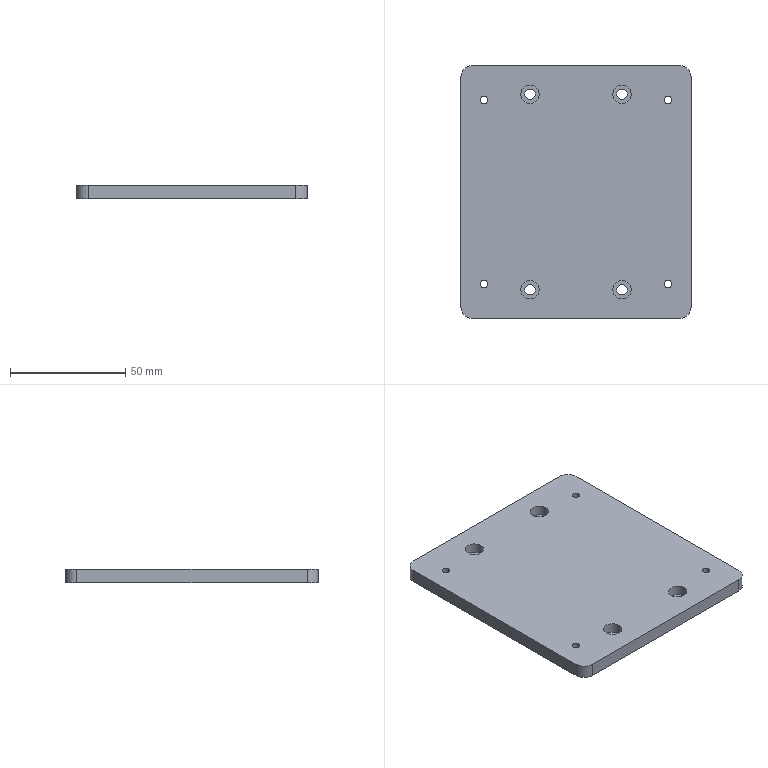Part | SolidWorks | features HoleWzd 2, Extrusion 1, Fillet 1 | 1 solid | 38 faces | box 100 x 110 x 6 mm | volume 64666 mm3 | cylinder 28 | plane 10 | commonest cylinder face diameters 3.3 x8 4.5 x8 8 x8 10 x4
STEP:
#1=CARTESIAN_POINT('',(-41.65,-40.,0.));
#2=VERTEX_POINT('',#1);
#3=CARTESIAN_POINT('',(-38.35,-40.,0.));
#4=VERTEX_POINT('',#3);
#5=CARTESIAN_POINT('',(-40.,-40.,0.));
#6=DIRECTION('',(0.,0.,1.));
#7=DIRECTION('',(1.,0.,0.));
#8=AXIS2_PLACEMENT_3D('',#5,#6,#7);
#9=CIRCLE('',#8,1.65);
#10=EDGE_CURVE('',#2,#4,#9,.T.);
#11=ORIENTED_EDGE('',*,*,#10,.F.);
#12=CARTESIAN_POINT('',(-41.65,-40.,6.));
#13=VERTEX_POINT('',#12);
#14=CARTESIAN_POINT('',(-41.65,-40.,6.));
#15=DIRECTION('',(0.,0.,1.));
#16=VECTOR('',#15,1000.);
#17=LINE('',#14,#16);
#18=EDGE_CURVE('',#2,#13,#17,.T.);
#19=ORIENTED_EDGE('',*,*,#18,.T.);
#20=CARTESIAN_POINT('',(-38.35,-40.,6.));
#21=VERTEX_POINT('',#20);
#22=CARTESIAN_POINT('',(-40.,-40.,6.));
#23=DIRECTION('',(0.,0.,1.));
#24=DIRECTION('',(1.,0.,0.));
#25=AXIS2_PLACEMENT_3D('',#22,#23,#24);
#26=CIRCLE('',#25,1.65);
#27=EDGE_CURVE('',#13,#21,#26,.T.);
#28=ORIENTED_EDGE('',*,*,#27,.T.);
#29=CARTESIAN_POINT('',(-38.35,-40.,6.));
#30=DIRECTION('',(0.,0.,1.));
#31=VECTOR('',#30,1000.);
#32=LINE('',#29,#31);
#33=EDGE_CURVE('',#4,#21,#32,.T.);
#34=ORIENTED_EDGE('',*,*,#33,.F.);
#35=EDGE_LOOP('',(#11,#19,#28,#34));
#36=FACE_OUTER_BOUND('',#35,.T.);
#37=CARTESIAN_POINT('',(-40.,-40.,6.));
#38=DIRECTION('',(0.,0.,1.));
#39=DIRECTION('',(1.,0.,0.));
#40=AXIS2_PLACEMENT_3D('',#37,#38,#39);
#41=CYLINDRICAL_SURFACE('',#40,1.65);
#42=ADVANCED_FACE('',(#36),#41,.F.);
#43=CARTESIAN_POINT('',(38.35,-40.,0.));
#44=VERTEX_POINT('',#43);
#45=CARTESIAN_POINT('',(41.65,-40.,0.));
#46=VERTEX_POINT('',#45);
#47=CARTESIAN_POINT('',(40.,-40.,0.));
#48=DIRECTION('',(0.,0.,1.));
#49=DIRECTION('',(1.,0.,0.));
#50=AXIS2_PLACEMENT_3D('',#47,#48,#49);
#51=CIRCLE('',#50,1.65);
#52=EDGE_CURVE('',#44,#46,#51,.T.);
#53=ORIENTED_EDGE('',*,*,#52,.F.);
#54=CARTESIAN_POINT('',(38.35,-40.,6.));
#55=VERTEX_POINT('',#54);
#56=CARTESIAN_POINT('',(38.35,-40.,6.));
#57=DIRECTION('',(0.,0.,1.));
#58=VECTOR('',#57,1000.);
#59=LINE('',#56,#58);
#60=EDGE_CURVE('',#44,#55,#59,.T.);
#61=ORIENTED_EDGE('',*,*,#60,.T.);
#62=CARTESIAN_POINT('',(41.65,-40.,6.));
#63=VERTEX_POINT('',#62);
#64=CARTESIAN_POINT('',(40.,-40.,6.));
#65=DIRECTION('',(0.,0.,1.));
#66=DIRECTION('',(1.,0.,0.));
#67=AXIS2_PLACEMENT_3D('',#64,#65,#66);
#68=CIRCLE('',#67,1.65);
#69=EDGE_CURVE('',#55,#63,#68,.T.);
#70=ORIENTED_EDGE('',*,*,#69,.T.);
#71=CARTESIAN_POINT('',(41.65,-40.,6.));
#72=DIRECTION('',(0.,0.,1.));
#73=VECTOR('',#72,1000.);
#74=LINE('',#71,#73);
#75=EDGE_CURVE('',#46,#63,#74,.T.);
#76=ORIENTED_EDGE('',*,*,#75,.F.);
#77=EDGE_LOOP('',(#53,#61,#70,#76));
#78=FACE_OUTER_BOUND('',#77,.T.);
#79=CARTESIAN_POINT('',(40.,-40.,6.));
#80=DIRECTION('',(0.,0.,1.));
#81=DIRECTION('',(1.,0.,0.));
#82=AXIS2_PLACEMENT_3D('',#79,#80,#81);
#83=CYLINDRICAL_SURFACE('',#82,1.65);
#84=ADVANCED_FACE('',(#78),#83,.F.);
#85=CARTESIAN_POINT('',(38.35,40.,0.));
#86=VERTEX_POINT('',#85);
#87=CARTESIAN_POINT('',(41.65,40.,0.));
#88=VERTEX_POINT('',#87);
#89=CARTESIAN_POINT('',(40.,40.,0.));
#90=DIRECTION('',(0.,0.,1.));
#91=DIRECTION('',(1.,0.,0.));
#92=AXIS2_PLACEMENT_3D('',#89,#90,#91);
#93=CIRCLE('',#92,1.65);
#94=EDGE_CURVE('',#86,#88,#93,.T.);
#95=ORIENTED_EDGE('',*,*,#94,.F.);
#96=CARTESIAN_POINT('',(38.35,40.,6.));
#97=VERTEX_POINT('',#96);
#98=CARTESIAN_POINT('',(38.35,40.,6.));
#99=DIRECTION('',(0.,0.,1.));
#100=VECTOR('',#99,1000.);
#101=LINE('',#98,#100);
#102=EDGE_CURVE('',#86,#97,#101,.T.);
#103=ORIENTED_EDGE('',*,*,#102,.T.);
#104=CARTESIAN_POINT('',(41.65,40.,6.));
#105=VERTEX_POINT('',#104);
#106=CARTESIAN_POINT('',(40.,40.,6.));
#107=DIRECTION('',(0.,0.,1.));
#108=DIRECTION('',(1.,0.,0.));
#109=AXIS2_PLACEMENT_3D('',#106,#107,#108);
#110=CIRCLE('',#109,1.65);
#111=EDGE_CURVE('',#97,#105,#110,.T.);
#112=ORIENTED_EDGE('',*,*,#111,.T.);
#113=CARTESIAN_POINT('',(41.65,40.,6.));
#114=DIRECTION('',(0.,0.,1.));
#115=VECTOR('',#114,1000.);
#116=LINE('',#113,#115);
#117=EDGE_CURVE('',#88,#105,#116,.T.);
#118=ORIENTED_EDGE('',*,*,#117,.F.);
#119=EDGE_LOOP('',(#95,#103,#112,#118));
#120=FACE_OUTER_BOUND('',#119,.T.);
#121=CARTESIAN_POINT('',(40.,40.,6.));
#122=DIRECTION('',(0.,0.,1.));
#123=DIRECTION('',(1.,0.,0.));
#124=AXIS2_PLACEMENT_3D('',#121,#122,#123);
#125=CYLINDRICAL_SURFACE('',#124,1.65);
#126=ADVANCED_FACE('',(#120),#125,.F.);
#127=CARTESIAN_POINT('',(-41.65,40.,0.));
#128=VERTEX_POINT('',#127);
#129=CARTESIAN_POINT('',(-38.35,40.,0.));
#130=VERTEX_POINT('',#129);
#131=CARTESIAN_POINT('',(-40.,40.,0.));
#132=DIRECTION('',(0.,0.,1.));
#133=DIRECTION('',(1.,0.,0.));
#134=AXIS2_PLACEMENT_3D('',#131,#132,#133);
#135=CIRCLE('',#134,1.65);
#136=EDGE_CURVE('',#128,#130,#135,.T.);
#137=ORIENTED_EDGE('',*,*,#136,.F.);
#138=CARTESIAN_POINT('',(-41.65,40.,6.));
#139=VERTEX_POINT('',#138);
#140=CARTESIAN_POINT('',(-41.65,40.,6.));
#141=DIRECTION('',(0.,0.,1.));
#142=VECTOR('',#141,1000.);
#143=LINE('',#140,#142);
#144=EDGE_CURVE('',#128,#139,#143,.T.);
#145=ORIENTED_EDGE('',*,*,#144,.T.);
#146=CARTESIAN_POINT('',(-38.35,40.,6.));
#147=VERTEX_POINT('',#146);
#148=CARTESIAN_POINT('',(-40.,40.,6.));
#149=DIRECTION('',(0.,0.,1.));
#150=DIRECTION('',(1.,0.,0.));
#151=AXIS2_PLACEMENT_3D('',#148,#149,#150);
#152=CIRCLE('',#151,1.65);
#153=EDGE_CURVE('',#139,#147,#152,.T.);
#154=ORIENTED_EDGE('',*,*,#153,.T.);
#155=CARTESIAN_POINT('',(-38.35,40.,6.));
#156=DIRECTION('',(0.,0.,1.));
#157=VECTOR('',#156,1000.);
#158=LINE('',#155,#157);
#159=EDGE_CURVE('',#130,#147,#158,.T.);
#160=ORIENTED_EDGE('',*,*,#159,.F.);
#161=EDGE_LOOP('',(#137,#145,#154,#160));
#162=FACE_OUTER_BOUND('',#161,.T.);
#163=CARTESIAN_POINT('',(-40.,40.,6.));
#164=DIRECTION('',(0.,0.,1.));
#165=DIRECTION('',(1.,0.,0.));
#166=AXIS2_PLACEMENT_3D('',#163,#164,#165);
#167=CYLINDRICAL_SURFACE('',#166,1.65);
#168=ADVANCED_FACE('',(#162),#167,.F.);
#169=CARTESIAN_POINT('',(-24.,42.5,1.5));
#170=VERTEX_POINT('',#169);
#171=CARTESIAN_POINT('',(-16.,42.5,1.5));
#172=VERTEX_POINT('',#171);
#173=CARTESIAN_POINT('',(-20.,42.5,1.5));
#174=DIRECTION('',(0.,0.,1.));
#175=DIRECTION('',(1.,0.,0.));
#176=AXIS2_PLACEMENT_3D('',#173,#174,#175);
#177=CIRCLE('',#176,4.);
#178=EDGE_CURVE('',#170,#172,#177,.T.);
#179=ORIENTED_EDGE('',*,*,#178,.F.);
#180=CARTESIAN_POINT('',(-24.,42.5,6.));
#181=VERTEX_POINT('',#180);
#182=CARTESIAN_POINT('',(-24.,42.5,6.));
#183=DIRECTION('',(0.,0.,1.));
#184=VECTOR('',#183,1000.);
#185=LINE('',#182,#184);
#186=EDGE_CURVE('',#170,#181,#185,.T.);
#187=ORIENTED_EDGE('',*,*,#186,.T.);
#188=CARTESIAN_POINT('',(-16.,42.5,6.));
#189=VERTEX_POINT('',#188);
#190=CARTESIAN_POINT('',(-20.,42.5,6.));
#191=DIRECTION('',(0.,0.,1.));
#192=DIRECTION('',(1.,0.,0.));
#193=AXIS2_PLACEMENT_3D('',#190,#191,#192);
#194=CIRCLE('',#193,4.);
#195=EDGE_CURVE('',#181,#189,#194,.T.);
#196=ORIENTED_EDGE('',*,*,#195,.T.);
#197=CARTESIAN_POINT('',(-16.,42.5,6.));
#198=DIRECTION('',(0.,0.,1.));
#199=VECTOR('',#198,1000.);
#200=LINE('',#197,#199);
#201=EDGE_CURVE('',#172,#189,#200,.T.);
#202=ORIENTED_EDGE('',*,*,#201,.F.);
#203=EDGE_LOOP('',(#179,#187,#196,#202));
#204=FACE_OUTER_BOUND('',#203,.T.);
#205=CARTESIAN_POINT('',(-20.,42.5,6.));
#206=DIRECTION('',(0.,0.,1.));
#207=DIRECTION('',(1.,0.,0.));
#208=AXIS2_PLACEMENT_3D('',#205,#206,#207);
#209=CYLINDRICAL_SURFACE('',#208,4.);
#210=ADVANCED_FACE('',(#204),#209,.F.);
#211=CARTESIAN_POINT('',(-22.25,42.5,0.));
#212=VERTEX_POINT('',#211);
#213=CARTESIAN_POINT('',(-17.75,42.5,0.));
#214=VERTEX_POINT('',#213);
#215=CARTESIAN_POINT('',(-20.,42.5,0.));
#216=DIRECTION('',(0.,0.,1.));
#217=DIRECTION('',(1.,0.,0.));
#218=AXIS2_PLACEMENT_3D('',#215,#216,#217);
#219=CIRCLE('',#218,2.25);
#220=EDGE_CURVE('',#212,#214,#219,.T.);
#221=ORIENTED_EDGE('',*,*,#220,.F.);
#222=CARTESIAN_POINT('',(-22.25,42.5,1.5));
#223=VERTEX_POINT('',#222);
#224=CARTESIAN_POINT('',(-22.25,42.5,6.));
#225=DIRECTION('',(0.,0.,1.));
#226=VECTOR('',#225,1000.);
#227=LINE('',#224,#226);
#228=EDGE_CURVE('',#212,#223,#227,.T.);
#229=ORIENTED_EDGE('',*,*,#228,.T.);
#230=CARTESIAN_POINT('',(-17.75,42.5,1.5));
#231=VERTEX_POINT('',#230);
#232=CARTESIAN_POINT('',(-20.,42.5,1.5));
#233=DIRECTION('',(0.,0.,1.));
#234=DIRECTION('',(1.,0.,0.));
#235=AXIS2_PLACEMENT_3D('',#232,#233,#234);
#236=CIRCLE('',#235,2.25);
#237=EDGE_CURVE('',#223,#231,#236,.T.);
#238=ORIENTED_EDGE('',*,*,#237,.T.);
#239=CARTESIAN_POINT('',(-17.75,42.5,6.));
#240=DIRECTION('',(0.,0.,1.));
#241=VECTOR('',#240,1000.);
#242=LINE('',#239,#241);
#243=EDGE_CURVE('',#214,#231,#242,.T.);
#244=ORIENTED_EDGE('',*,*,#243,.F.);
#245=EDGE_LOOP('',(#221,#229,#238,#244));
#246=FACE_OUTER_BOUND('',#245,.T.);
#247=CARTESIAN_POINT('',(-20.,42.5,6.));
#248=DIRECTION('',(0.,0.,1.));
#249=DIRECTION('',(1.,0.,0.));
#250=AXIS2_PLACEMENT_3D('',#247,#248,#249);
#251=CYLINDRICAL_SURFACE('',#250,2.25);
#252=ADVANCED_FACE('',(#246),#251,.F.);
#253=CARTESIAN_POINT('',(16.,42.5,1.5));
#254=VERTEX_POINT('',#253);
#255=CARTESIAN_POINT('',(24.,42.5,1.5));
#256=VERTEX_POINT('',#255);
#257=CARTESIAN_POINT('',(20.,42.5,1.5));
#258=DIRECTION('',(0.,0.,1.));
#259=DIRECTION('',(1.,0.,0.));
#260=AXIS2_PLACEMENT_3D('',#257,#258,#259);
#261=CIRCLE('',#260,4.);
#262=EDGE_CURVE('',#254,#256,#261,.T.);
#263=ORIENTED_EDGE('',*,*,#262,.F.);
#264=CARTESIAN_POINT('',(16.,42.5,6.));
#265=VERTEX_POINT('',#264);
#266=CARTESIAN_POINT('',(16.,42.5,6.));
#267=DIRECTION('',(0.,0.,1.));
#268=VECTOR('',#267,1000.);
#269=LINE('',#266,#268);
#270=EDGE_CURVE('',#254,#265,#269,.T.);
#271=ORIENTED_EDGE('',*,*,#270,.T.);
#272=CARTESIAN_POINT('',(24.,42.5,6.));
#273=VERTEX_POINT('',#272);
#274=CARTESIAN_POINT('',(20.,42.5,6.));
#275=DIRECTION('',(0.,0.,1.));
#276=DIRECTION('',(1.,0.,0.));
#277=AXIS2_PLACEMENT_3D('',#274,#275,#276);
#278=CIRCLE('',#277,4.);
#279=EDGE_CURVE('',#265,#273,#278,.T.);
#280=ORIENTED_EDGE('',*,*,#279,.T.);
#281=CARTESIAN_POINT('',(24.,42.5,6.));
#282=DIRECTION('',(0.,0.,1.));
#283=VECTOR('',#282,1000.);
#284=LINE('',#281,#283);
#285=EDGE_CURVE('',#256,#273,#284,.T.);
#286=ORIENTED_EDGE('',*,*,#285,.F.);
#287=EDGE_LOOP('',(#263,#271,#280,#286));
#288=FACE_OUTER_BOUND('',#287,.T.);
#289=CARTESIAN_POINT('',(20.,42.5,6.));
#290=DIRECTION('',(0.,0.,1.));
#291=DIRECTION('',(1.,0.,0.));
#292=AXIS2_PLACEMENT_3D('',#289,#290,#291);
#293=CYLINDRICAL_SURFACE('',#292,4.);
#294=ADVANCED_FACE('',(#288),#293,.F.);
#295=CARTESIAN_POINT('',(17.75,42.5,0.));
#296=VERTEX_POINT('',#295);
#297=CARTESIAN_POINT('',(22.25,42.5,0.));
#298=VERTEX_POINT('',#297);
#299=CARTESIAN_POINT('',(20.,42.5,0.));
#300=DIRECTION('',(0.,0.,1.));
#301=DIRECTION('',(1.,0.,0.));
#302=AXIS2_PLACEMENT_3D('',#299,#300,#301);
#303=CIRCLE('',#302,2.25);
#304=EDGE_CURVE('',#296,#298,#303,.T.);
#305=ORIENTED_EDGE('',*,*,#304,.F.);
#306=CARTESIAN_POINT('',(17.75,42.5,1.5));
#307=VERTEX_POINT('',#306);
#308=CARTESIAN_POINT('',(17.75,42.5,6.));
#309=DIRECTION('',(0.,0.,1.));
#310=VECTOR('',#309,1000.);
#311=LINE('',#308,#310);
#312=EDGE_CURVE('',#296,#307,#311,.T.);
#313=ORIENTED_EDGE('',*,*,#312,.T.);
#314=CARTESIAN_POINT('',(22.25,42.5,1.5));
#315=VERTEX_POINT('',#314);
#316=CARTESIAN_POINT('',(20.,42.5,1.5));
#317=DIRECTION('',(0.,0.,1.));
#318=DIRECTION('',(1.,0.,0.));
#319=AXIS2_PLACEMENT_3D('',#316,#317,#318);
#320=CIRCLE('',#319,2.25);
#321=EDGE_CURVE('',#307,#315,#320,.T.);
#322=ORIENTED_EDGE('',*,*,#321,.T.);
#323=CARTESIAN_POINT('',(22.25,42.5,6.));
#324=DIRECTION('',(0.,0.,1.));
#325=VECTOR('',#324,1000.);
#326=LINE('',#323,#325);
#327=EDGE_CURVE('',#298,#315,#326,.T.);
#328=ORIENTED_EDGE('',*,*,#327,.F.);
#329=EDGE_LOOP('',(#305,#313,#322,#328));
#330=FACE_OUTER_BOUND('',#329,.T.);
#331=CARTESIAN_POINT('',(20.,42.5,6.));
#332=DIRECTION('',(0.,0.,1.));
#333=DIRECTION('',(1.,0.,0.));
#334=AXIS2_PLACEMENT_3D('',#331,#332,#333);
#335=CYLINDRICAL_SURFACE('',#334,2.25);
#336=ADVANCED_FACE('',(#330),#335,.F.);
#337=CARTESIAN_POINT('',(16.,-42.5,1.5));
#338=VERTEX_POINT('',#337);
#339=CARTESIAN_POINT('',(24.,-42.5,1.5));
#340=VERTEX_POINT('',#339);
#341=CARTESIAN_POINT('',(20.,-42.5,1.5));
#342=DIRECTION('',(0.,0.,1.));
#343=DIRECTION('',(1.,0.,0.));
#344=AXIS2_PLACEMENT_3D('',#341,#342,#343);
#345=CIRCLE('',#344,4.);
#346=EDGE_CURVE('',#338,#340,#345,.T.);
#347=ORIENTED_EDGE('',*,*,#346,.F.);
#348=CARTESIAN_POINT('',(16.,-42.5,6.));
#349=VERTEX_POINT('',#348);
#350=CARTESIAN_POINT('',(16.,-42.5,6.));
#351=DIRECTION('',(0.,0.,1.));
#352=VECTOR('',#351,1000.);
#353=LINE('',#350,#352);
#354=EDGE_CURVE('',#338,#349,#353,.T.);
#355=ORIENTED_EDGE('',*,*,#354,.T.);
#356=CARTESIAN_POINT('',(24.,-42.5,6.));
#357=VERTEX_POINT('',#356);
#358=CARTESIAN_POINT('',(20.,-42.5,6.));
#359=DIRECTION('',(0.,0.,1.));
#360=DIRECTION('',(1.,0.,0.));
#361=AXIS2_PLACEMENT_3D('',#358,#359,#360);
#362=CIRCLE('',#361,4.);
#363=EDGE_CURVE('',#349,#357,#362,.T.);
#364=ORIENTED_EDGE('',*,*,#363,.T.);
#365=CARTESIAN_POINT('',(24.,-42.5,6.));
#366=DIRECTION('',(0.,0.,1.));
#367=VECTOR('',#366,1000.);
#368=LINE('',#365,#367);
#369=EDGE_CURVE('',#340,#357,#368,.T.);
#370=ORIENTED_EDGE('',*,*,#369,.F.);
#371=EDGE_LOOP('',(#347,#355,#364,#370));
#372=FACE_OUTER_BOUND('',#371,.T.);
#373=CARTESIAN_POINT('',(20.,-42.5,6.));
#374=DIRECTION('',(0.,0.,1.));
#375=DIRECTION('',(1.,0.,0.));
#376=AXIS2_PLACEMENT_3D('',#373,#374,#375);
#377=CYLINDRICAL_SURFACE('',#376,4.);
#378=ADVANCED_FACE('',(#372),#377,.F.);
#379=CARTESIAN_POINT('',(17.75,-42.5,0.));
#380=VERTEX_POINT('',#379);
#381=CARTESIAN_POINT('',(22.25,-42.5,0.));
#382=VERTEX_POINT('',#381);
#383=CARTESIAN_POINT('',(20.,-42.5,0.));
#384=DIRECTION('',(0.,0.,1.));
#385=DIRECTION('',(1.,0.,0.));
#386=AXIS2_PLACEMENT_3D('',#383,#384,#385);
#387=CIRCLE('',#386,2.25);
#388=EDGE_CURVE('',#380,#382,#387,.T.);
#389=ORIENTED_EDGE('',*,*,#388,.F.);
#390=CARTESIAN_POINT('',(17.75,-42.5,1.5));
#391=VERTEX_POINT('',#390);
#392=CARTESIAN_POINT('',(17.75,-42.5,6.));
#393=DIRECTION('',(0.,0.,1.));
#394=VECTOR('',#393,1000.);
#395=LINE('',#392,#394);
#396=EDGE_CURVE('',#380,#391,#395,.T.);
#397=ORIENTED_EDGE('',*,*,#396,.T.);
#398=CARTESIAN_POINT('',(22.25,-42.5,1.5));
#399=VERTEX_POINT('',#398);
#400=CARTESIAN_POINT('',(20.,-42.5,1.5));
#401=DIRECTION('',(0.,0.,1.));
#402=DIRECTION('',(1.,0.,0.));
#403=AXIS2_PLACEMENT_3D('',#400,#401,#402);
#404=CIRCLE('',#403,2.25);
#405=EDGE_CURVE('',#391,#399,#404,.T.);
#406=ORIENTED_EDGE('',*,*,#405,.T.);
#407=CARTESIAN_POINT('',(22.25,-42.5,6.));
#408=DIRECTION('',(0.,0.,1.));
#409=VECTOR('',#408,1000.);
#410=LINE('',#407,#409);
#411=EDGE_CURVE('',#382,#399,#410,.T.);
#412=ORIENTED_EDGE('',*,*,#411,.F.);
#413=EDGE_LOOP('',(#389,#397,#406,#412));
#414=FACE_OUTER_BOUND('',#413,.T.);
#415=CARTESIAN_POINT('',(20.,-42.5,6.));
#416=DIRECTION('',(0.,0.,1.));
#417=DIRECTION('',(1.,0.,0.));
#418=AXIS2_PLACEMENT_3D('',#415,#416,#417);
#419=CYLINDRICAL_SURFACE('',#418,2.25);
#420=ADVANCED_FACE('',(#414),#419,.F.);
#421=CARTESIAN_POINT('',(-24.,-42.5,1.5));
#422=VERTEX_POINT('',#421);
#423=CARTESIAN_POINT('',(-16.,-42.5,1.5));
#424=VERTEX_POINT('',#423);
#425=CARTESIAN_POINT('',(-20.,-42.5,1.5));
#426=DIRECTION('',(0.,0.,1.));
#427=DIRECTION('',(1.,0.,0.));
#428=AXIS2_PLACEMENT_3D('',#425,#426,#427);
#429=CIRCLE('',#428,4.);
#430=EDGE_CURVE('',#422,#424,#429,.T.);
#431=ORIENTED_EDGE('',*,*,#430,.F.);
#432=CARTESIAN_POINT('',(-24.,-42.5,6.));
#433=VERTEX_POINT('',#432);
#434=CARTESIAN_POINT('',(-24.,-42.5,6.));
#435=DIRECTION('',(0.,0.,1.));
#436=VECTOR('',#435,1000.);
#437=LINE('',#434,#436);
#438=EDGE_CURVE('',#422,#433,#437,.T.);
#439=ORIENTED_EDGE('',*,*,#438,.T.);
#440=CARTESIAN_POINT('',(-16.,-42.5,6.));
#441=VERTEX_POINT('',#440);
#442=CARTESIAN_POINT('',(-20.,-42.5,6.));
#443=DIRECTION('',(0.,0.,1.));
#444=DIRECTION('',(1.,0.,0.));
#445=AXIS2_PLACEMENT_3D('',#442,#443,#444);
#446=CIRCLE('',#445,4.);
#447=EDGE_CURVE('',#433,#441,#446,.T.);
#448=ORIENTED_EDGE('',*,*,#447,.T.);
#449=CARTESIAN_POINT('',(-16.,-42.5,6.));
#450=DIRECTION('',(0.,0.,1.));
#451=VECTOR('',#450,1000.);
#452=LINE('',#449,#451);
#453=EDGE_CURVE('',#424,#441,#452,.T.);
#454=ORIENTED_EDGE('',*,*,#453,.F.);
#455=EDGE_LOOP('',(#431,#439,#448,#454));
#456=FACE_OUTER_BOUND('',#455,.T.);
#457=CARTESIAN_POINT('',(-20.,-42.5,6.));
#458=DIRECTION('',(0.,0.,1.));
#459=DIRECTION('',(1.,0.,0.));
#460=AXIS2_PLACEMENT_3D('',#457,#458,#459);
#461=CYLINDRICAL_SURFACE('',#460,4.);
#462=ADVANCED_FACE('',(#456),#461,.F.);
#463=CARTESIAN_POINT('',(-22.25,-42.5,0.));
#464=VERTEX_POINT('',#463);
#465=CARTESIAN_POINT('',(-17.75,-42.5,0.));
#466=VERTEX_POINT('',#465);
#467=CARTESIAN_POINT('',(-20.,-42.5,0.));
#468=DIRECTION('',(0.,0.,1.));
#469=DIRECTION('',(1.,0.,0.));
#470=AXIS2_PLACEMENT_3D('',#467,#468,#469);
#471=CIRCLE('',#470,2.25);
#472=EDGE_CURVE('',#464,#466,#471,.T.);
#473=ORIENTED_EDGE('',*,*,#472,.F.);
#474=CARTESIAN_POINT('',(-22.25,-42.5,1.5));
#475=VERTEX_POINT('',#474);
#476=CARTESIAN_POINT('',(-22.25,-42.5,6.));
#477=DIRECTION('',(0.,0.,1.));
#478=VECTOR('',#477,1000.);
#479=LINE('',#476,#478);
#480=EDGE_CURVE('',#464,#475,#479,.T.);
#481=ORIENTED_EDGE('',*,*,#480,.T.);
#482=CARTESIAN_POINT('',(-17.75,-42.5,1.5));
#483=VERTEX_POINT('',#482);
#484=CARTESIAN_POINT('',(-20.,-42.5,1.5));
#485=DIRECTION('',(0.,0.,1.));
#486=DIRECTION('',(1.,0.,0.));
#487=AXIS2_PLACEMENT_3D('',#484,#485,#486);
#488=CIRCLE('',#487,2.25);
#489=EDGE_CURVE('',#475,#483,#488,.T.);
#490=ORIENTED_EDGE('',*,*,#489,.T.);
#491=CARTESIAN_POINT('',(-17.75,-42.5,6.));
#492=DIRECTION('',(0.,0.,1.));
#493=VECTOR('',#492,1000.);
#494=LINE('',#491,#493);
#495=EDGE_CURVE('',#466,#483,#494,.T.);
#496=ORIENTED_EDGE('',*,*,#495,.F.);
#497=EDGE_LOOP('',(#473,#481,#490,#496));
#498=FACE_OUTER_BOUND('',#497,.T.);
#499=CARTESIAN_POINT('',(-20.,-42.5,6.));
#500=DIRECTION('',(0.,0.,1.));
#501=DIRECTION('',(1.,0.,0.));
#502=AXIS2_PLACEMENT_3D('',#499,#500,#501);
#503=CYLINDRICAL_SURFACE('',#502,2.25);
#504=ADVANCED_FACE('',(#498),#503,.F.);
#505=CARTESIAN_POINT('',(40.,-40.,6.));
#506=DIRECTION('',(0.,0.,1.));
#507=DIRECTION('',(1.,0.,0.));
#508=AXIS2_PLACEMENT_3D('',#505,#506,#507);
#509=CIRCLE('',#508,1.65);
#510=EDGE_CURVE('',#63,#55,#509,.T.);
#511=ORIENTED_EDGE('',*,*,#510,.F.);
#512=ORIENTED_EDGE('',*,*,#69,.F.);
#513=EDGE_LOOP('',(#511,#512));
#514=FACE_BOUND('',#513,.T.);
#515=CARTESIAN_POINT('',(45.,55.,6.));
#516=VERTEX_POINT('',#515);
#517=CARTESIAN_POINT('',(-45.,55.,6.));
#518=VERTEX_POINT('',#517);
#519=CARTESIAN_POINT('',(-50.,55.,6.));
#520=DIRECTION('',(-1.,0.,0.));
#521=VECTOR('',#520,1000.);
#522=LINE('',#519,#521);
#523=EDGE_CURVE('',#516,#518,#522,.T.);
#524=ORIENTED_EDGE('',*,*,#523,.T.);
#525=CARTESIAN_POINT('',(-50.,50.,6.));
#526=VERTEX_POINT('',#525);
#527=CARTESIAN_POINT('',(-45.,50.,6.));
#528=DIRECTION('',(0.,0.,1.));
#529=DIRECTION('',(-1.,0.,0.));
#530=AXIS2_PLACEMENT_3D('',#527,#528,#529);
#531=CIRCLE('',#530,5.);
#532=EDGE_CURVE('',#518,#526,#531,.T.);
#533=ORIENTED_EDGE('',*,*,#532,.T.);
#534=CARTESIAN_POINT('',(-50.,-50.,6.));
#535=VERTEX_POINT('',#534);
#536=CARTESIAN_POINT('',(-50.,-55.,6.));
#537=DIRECTION('',(0.,-1.,0.));
#538=VECTOR('',#537,1000.);
#539=LINE('',#536,#538);
#540=EDGE_CURVE('',#526,#535,#539,.T.);
#541=ORIENTED_EDGE('',*,*,#540,.T.);
#542=CARTESIAN_POINT('',(-45.,-55.,6.));
#543=VERTEX_POINT('',#542);
#544=CARTESIAN_POINT('',(-45.,-50.,6.));
#545=DIRECTION('',(0.,0.,1.));
#546=DIRECTION('',(-1.,0.,0.));
#547=AXIS2_PLACEMENT_3D('',#544,#545,#546);
#548=CIRCLE('',#547,5.);
#549=EDGE_CURVE('',#535,#543,#548,.T.);
#550=ORIENTED_EDGE('',*,*,#549,.T.);
#551=CARTESIAN_POINT('',(45.,-55.,6.));
#552=VERTEX_POINT('',#551);
#553=CARTESIAN_POINT('',(-50.,-55.,6.));
#554=DIRECTION('',(1.,0.,0.));
#555=VECTOR('',#554,1000.);
#556=LINE('',#553,#555);
#557=EDGE_CURVE('',#543,#552,#556,.T.);
#558=ORIENTED_EDGE('',*,*,#557,.T.);
#559=CARTESIAN_POINT('',(50.,-50.,6.));
#560=VERTEX_POINT('',#559);
#561=CARTESIAN_POINT('',(45.,-50.,6.));
#562=DIRECTION('',(0.,0.,1.));
#563=DIRECTION('',(-1.,0.,0.));
#564=AXIS2_PLACEMENT_3D('',#561,#562,#563);
#565=CIRCLE('',#564,5.);
#566=EDGE_CURVE('',#552,#560,#565,.T.);
#567=ORIENTED_EDGE('',*,*,#566,.T.);
#568=CARTESIAN_POINT('',(50.,50.,6.));
#569=VERTEX_POINT('',#568);
#570=CARTESIAN_POINT('',(50.,-55.,6.));
#571=DIRECTION('',(0.,1.,0.));
#572=VECTOR('',#571,1000.);
#573=LINE('',#570,#572);
#574=EDGE_CURVE('',#560,#569,#573,.T.);
#575=ORIENTED_EDGE('',*,*,#574,.T.);
#576=CARTESIAN_POINT('',(45.,50.,6.));
#577=DIRECTION('',(0.,0.,1.));
#578=DIRECTION('',(-1.,0.,0.));
#579=AXIS2_PLACEMENT_3D('',#576,#577,#578);
#580=CIRCLE('',#579,5.);
#581=EDGE_CURVE('',#569,#516,#580,.T.);
#582=ORIENTED_EDGE('',*,*,#581,.T.);
#583=EDGE_LOOP('',(#524,#533,#541,#550,#558,#567,#575,#582));
#584=FACE_OUTER_BOUND('',#583,.T.);
#585=CARTESIAN_POINT('',(-20.,-42.5,6.));
#586=DIRECTION('',(0.,0.,1.));
#587=DIRECTION('',(1.,0.,0.));
#588=AXIS2_PLACEMENT_3D('',#585,#586,#587);
#589=CIRCLE('',#588,4.);
#590=EDGE_CURVE('',#441,#433,#589,.T.);
#591=ORIENTED_EDGE('',*,*,#590,.F.);
#592=ORIENTED_EDGE('',*,*,#447,.F.);
#593=EDGE_LOOP('',(#591,#592));
#594=FACE_BOUND('',#593,.T.);
#595=CARTESIAN_POINT('',(20.,-42.5,6.));
#596=DIRECTION('',(0.,0.,1.));
#597=DIRECTION('',(1.,0.,0.));
#598=AXIS2_PLACEMENT_3D('',#595,#596,#597);
#599=CIRCLE('',#598,4.);
#600=EDGE_CURVE('',#357,#349,#599,.T.);
#601=ORIENTED_EDGE('',*,*,#600,.F.);
#602=ORIENTED_EDGE('',*,*,#363,.F.);
#603=EDGE_LOOP('',(#601,#602));
#604=FACE_BOUND('',#603,.T.);
#605=CARTESIAN_POINT('',(20.,42.5,6.));
#606=DIRECTION('',(0.,0.,1.));
#607=DIRECTION('',(1.,0.,0.));
#608=AXIS2_PLACEMENT_3D('',#605,#606,#607);
#609=CIRCLE('',#608,4.);
#610=EDGE_CURVE('',#273,#265,#609,.T.);
#611=ORIENTED_EDGE('',*,*,#610,.F.);
#612=ORIENTED_EDGE('',*,*,#279,.F.);
#613=EDGE_LOOP('',(#611,#612));
#614=FACE_BOUND('',#613,.T.);
#615=CARTESIAN_POINT('',(-20.,42.5,6.));
#616=DIRECTION('',(0.,0.,1.));
#617=DIRECTION('',(1.,0.,0.));
#618=AXIS2_PLACEMENT_3D('',#615,#616,#617);
#619=CIRCLE('',#618,4.);
#620=EDGE_CURVE('',#189,#181,#619,.T.);
#621=ORIENTED_EDGE('',*,*,#620,.F.);
#622=ORIENTED_EDGE('',*,*,#195,.F.);
#623=EDGE_LOOP('',(#621,#622));
#624=FACE_BOUND('',#623,.T.);
#625=CARTESIAN_POINT('',(-40.,40.,6.));
#626=DIRECTION('',(0.,0.,1.));
#627=DIRECTION('',(1.,0.,0.));
#628=AXIS2_PLACEMENT_3D('',#625,#626,#627);
#629=CIRCLE('',#628,1.65);
#630=EDGE_CURVE('',#147,#139,#629,.T.);
#631=ORIENTED_EDGE('',*,*,#630,.F.);
#632=ORIENTED_EDGE('',*,*,#153,.F.);
#633=EDGE_LOOP('',(#631,#632));
#634=FACE_BOUND('',#633,.T.);
#635=CARTESIAN_POINT('',(40.,40.,6.));
#636=DIRECTION('',(0.,0.,1.));
#637=DIRECTION('',(1.,0.,0.));
#638=AXIS2_PLACEMENT_3D('',#635,#636,#637);
#639=CIRCLE('',#638,1.65);
#640=EDGE_CURVE('',#105,#97,#639,.T.);
#641=ORIENTED_EDGE('',*,*,#640,.F.);
#642=ORIENTED_EDGE('',*,*,#111,.F.);
#643=EDGE_LOOP('',(#641,#642));
#644=FACE_BOUND('',#643,.T.);
#645=CARTESIAN_POINT('',(-40.,-40.,6.));
#646=DIRECTION('',(0.,0.,1.));
#647=DIRECTION('',(1.,0.,0.));
#648=AXIS2_PLACEMENT_3D('',#645,#646,#647);
#649=CIRCLE('',#648,1.65);
#650=EDGE_CURVE('',#21,#13,#649,.T.);
#651=ORIENTED_EDGE('',*,*,#650,.F.);
#652=ORIENTED_EDGE('',*,*,#27,.F.);
#653=EDGE_LOOP('',(#651,#652));
#654=FACE_BOUND('',#653,.T.);
#655=CARTESIAN_POINT('',(0.,0.,6.));
#656=DIRECTION('',(0.,0.,-1.));
#657=DIRECTION('',(-1.,0.,0.));
#658=AXIS2_PLACEMENT_3D('',#655,#656,#657);
#659=PLANE('',#658);
#660=ADVANCED_FACE('',(#514,#584,#594,#604,#614,#624,#634,#644,#654),#659,.F.);
#661=CARTESIAN_POINT('',(40.,40.,0.));
#662=DIRECTION('',(0.,0.,1.));
#663=DIRECTION('',(1.,0.,0.));
#664=AXIS2_PLACEMENT_3D('',#661,#662,#663);
#665=CIRCLE('',#664,1.65);
#666=EDGE_CURVE('',#88,#86,#665,.T.);
#667=ORIENTED_EDGE('',*,*,#666,.T.);
#668=ORIENTED_EDGE('',*,*,#94,.T.);
#669=EDGE_LOOP('',(#667,#668));
#670=FACE_BOUND('',#669,.T.);
#671=CARTESIAN_POINT('',(-40.,40.,0.));
#672=DIRECTION('',(0.,0.,1.));
#673=DIRECTION('',(1.,0.,0.));
#674=AXIS2_PLACEMENT_3D('',#671,#672,#673);
#675=CIRCLE('',#674,1.65);
#676=EDGE_CURVE('',#130,#128,#675,.T.);
#677=ORIENTED_EDGE('',*,*,#676,.T.);
#678=ORIENTED_EDGE('',*,*,#136,.T.);
#679=EDGE_LOOP('',(#677,#678));
#680=FACE_BOUND('',#679,.T.);
#681=CARTESIAN_POINT('',(20.,42.5,0.));
#682=DIRECTION('',(0.,0.,1.));
#683=DIRECTION('',(1.,0.,0.));
#684=AXIS2_PLACEMENT_3D('',#681,#682,#683);
#685=CIRCLE('',#684,2.25);
#686=EDGE_CURVE('',#298,#296,#685,.T.);
#687=ORIENTED_EDGE('',*,*,#686,.T.);
#688=ORIENTED_EDGE('',*,*,#304,.T.);
#689=EDGE_LOOP('',(#687,#688));
#690=FACE_BOUND('',#689,.T.);
#691=CARTESIAN_POINT('',(20.,-42.5,0.));
#692=DIRECTION('',(0.,0.,1.));
#693=DIRECTION('',(1.,0.,0.));
#694=AXIS2_PLACEMENT_3D('',#691,#692,#693);
#695=CIRCLE('',#694,2.25);
#696=EDGE_CURVE('',#382,#380,#695,.T.);
#697=ORIENTED_EDGE('',*,*,#696,.T.);
#698=ORIENTED_EDGE('',*,*,#388,.T.);
#699=EDGE_LOOP('',(#697,#698));
#700=FACE_BOUND('',#699,.T.);
#701=CARTESIAN_POINT('',(-20.,-42.5,0.));
#702=DIRECTION('',(0.,0.,1.));
#703=DIRECTION('',(1.,0.,0.));
#704=AXIS2_PLACEMENT_3D('',#701,#702,#703);
#705=CIRCLE('',#704,2.25);
#706=EDGE_CURVE('',#466,#464,#705,.T.);
#707=ORIENTED_EDGE('',*,*,#706,.T.);
#708=ORIENTED_EDGE('',*,*,#472,.T.);
#709=EDGE_LOOP('',(#707,#708));
#710=FACE_BOUND('',#709,.T.);
#711=CARTESIAN_POINT('',(-50.,50.,0.));
#712=VERTEX_POINT('',#711);
#713=CARTESIAN_POINT('',(-50.,-50.,0.));
#714=VERTEX_POINT('',#713);
#715=CARTESIAN_POINT('',(-50.,-55.,0.));
#716=DIRECTION('',(0.,-1.,0.));
#717=VECTOR('',#716,1000.);
#718=LINE('',#715,#717);
#719=EDGE_CURVE('',#712,#714,#718,.T.);
#720=ORIENTED_EDGE('',*,*,#719,.F.);
#721=CARTESIAN_POINT('',(-45.,55.,0.));
#722=VERTEX_POINT('',#721);
#723=CARTESIAN_POINT('',(-45.,50.,0.));
#724=DIRECTION('',(0.,0.,-1.));
#725=DIRECTION('',(-1.,0.,0.));
#726=AXIS2_PLACEMENT_3D('',#723,#724,#725);
#727=CIRCLE('',#726,5.);
#728=EDGE_CURVE('',#712,#722,#727,.T.);
#729=ORIENTED_EDGE('',*,*,#728,.T.);
#730=CARTESIAN_POINT('',(45.,55.,0.));
#731=VERTEX_POINT('',#730);
#732=CARTESIAN_POINT('',(-50.,55.,0.));
#733=DIRECTION('',(-1.,0.,0.));
#734=VECTOR('',#733,1000.);
#735=LINE('',#732,#734);
#736=EDGE_CURVE('',#731,#722,#735,.T.);
#737=ORIENTED_EDGE('',*,*,#736,.F.);
#738=CARTESIAN_POINT('',(50.,50.,0.));
#739=VERTEX_POINT('',#738);
#740=CARTESIAN_POINT('',(45.,50.,0.));
#741=DIRECTION('',(0.,0.,-1.));
#742=DIRECTION('',(-1.,0.,0.));
#743=AXIS2_PLACEMENT_3D('',#740,#741,#742);
#744=CIRCLE('',#743,5.);
#745=EDGE_CURVE('',#731,#739,#744,.T.);
#746=ORIENTED_EDGE('',*,*,#745,.T.);
#747=CARTESIAN_POINT('',(50.,-50.,0.));
#748=VERTEX_POINT('',#747);
#749=CARTESIAN_POINT('',(50.,-55.,0.));
#750=DIRECTION('',(0.,1.,0.));
#751=VECTOR('',#750,1000.);
#752=LINE('',#749,#751);
#753=EDGE_CURVE('',#748,#739,#752,.T.);
#754=ORIENTED_EDGE('',*,*,#753,.F.);
#755=CARTESIAN_POINT('',(45.,-55.,0.));
#756=VERTEX_POINT('',#755);
#757=CARTESIAN_POINT('',(45.,-50.,0.));
#758=DIRECTION('',(0.,0.,-1.));
#759=DIRECTION('',(-1.,0.,0.));
#760=AXIS2_PLACEMENT_3D('',#757,#758,#759);
#761=CIRCLE('',#760,5.);
#762=EDGE_CURVE('',#748,#756,#761,.T.);
#763=ORIENTED_EDGE('',*,*,#762,.T.);
#764=CARTESIAN_POINT('',(-45.,-55.,0.));
#765=VERTEX_POINT('',#764);
#766=CARTESIAN_POINT('',(-50.,-55.,0.));
#767=DIRECTION('',(1.,0.,0.));
#768=VECTOR('',#767,1000.);
#769=LINE('',#766,#768);
#770=EDGE_CURVE('',#765,#756,#769,.T.);
#771=ORIENTED_EDGE('',*,*,#770,.F.);
#772=CARTESIAN_POINT('',(-45.,-50.,0.));
#773=DIRECTION('',(0.,0.,-1.));
#774=DIRECTION('',(-1.,0.,0.));
#775=AXIS2_PLACEMENT_3D('',#772,#773,#774);
#776=CIRCLE('',#775,5.);
#777=EDGE_CURVE('',#765,#714,#776,.T.);
#778=ORIENTED_EDGE('',*,*,#777,.T.);
#779=EDGE_LOOP('',(#720,#729,#737,#746,#754,#763,#771,#778));
#780=FACE_OUTER_BOUND('',#779,.T.);
#781=CARTESIAN_POINT('',(-20.,42.5,0.));
#782=DIRECTION('',(0.,0.,1.));
#783=DIRECTION('',(1.,0.,0.));
#784=AXIS2_PLACEMENT_3D('',#781,#782,#783);
#785=CIRCLE('',#784,2.25);
#786=EDGE_CURVE('',#214,#212,#785,.T.);
#787=ORIENTED_EDGE('',*,*,#786,.T.);
#788=ORIENTED_EDGE('',*,*,#220,.T.);
#789=EDGE_LOOP('',(#787,#788));
#790=FACE_BOUND('',#789,.T.);
#791=CARTESIAN_POINT('',(40.,-40.,0.));
#792=DIRECTION('',(0.,0.,1.));
#793=DIRECTION('',(1.,0.,0.));
#794=AXIS2_PLACEMENT_3D('',#791,#792,#793);
#795=CIRCLE('',#794,1.65);
#796=EDGE_CURVE('',#46,#44,#795,.T.);
#797=ORIENTED_EDGE('',*,*,#796,.T.);
#798=ORIENTED_EDGE('',*,*,#52,.T.);
#799=EDGE_LOOP('',(#797,#798));
#800=FACE_BOUND('',#799,.T.);
#801=CARTESIAN_POINT('',(-40.,-40.,0.));
#802=DIRECTION('',(0.,0.,1.));
#803=DIRECTION('',(1.,0.,0.));
#804=AXIS2_PLACEMENT_3D('',#801,#802,#803);
#805=CIRCLE('',#804,1.65);
#806=EDGE_CURVE('',#4,#2,#805,.T.);
#807=ORIENTED_EDGE('',*,*,#806,.T.);
#808=ORIENTED_EDGE('',*,*,#10,.T.);
#809=EDGE_LOOP('',(#807,#808));
#810=FACE_BOUND('',#809,.T.);
#811=CARTESIAN_POINT('',(0.,0.,0.));
#812=DIRECTION('',(0.,0.,-1.));
#813=DIRECTION('',(-1.,0.,0.));
#814=AXIS2_PLACEMENT_3D('',#811,#812,#813);
#815=PLANE('',#814);
#816=ADVANCED_FACE('',(#670,#680,#690,#700,#710,#780,#790,#800,#810),#815,.T.);
#817=ORIENTED_EDGE('',*,*,#574,.F.);
#818=CARTESIAN_POINT('',(50.,-50.,6.));
#819=DIRECTION('',(0.,0.,-1.));
#820=VECTOR('',#819,1000.);
#821=LINE('',#818,#820);
#822=EDGE_CURVE('',#560,#748,#821,.T.);
#823=ORIENTED_EDGE('',*,*,#822,.T.);
#824=ORIENTED_EDGE('',*,*,#753,.T.);
#825=CARTESIAN_POINT('',(50.,50.,6.));
#826=DIRECTION('',(0.,0.,1.));
#827=VECTOR('',#826,1000.);
#828=LINE('',#825,#827);
#829=EDGE_CURVE('',#739,#569,#828,.T.);
#830=ORIENTED_EDGE('',*,*,#829,.T.);
#831=EDGE_LOOP('',(#817,#823,#824,#830));
#832=FACE_OUTER_BOUND('',#831,.T.);
#833=CARTESIAN_POINT('',(50.,-55.,6.));
#834=DIRECTION('',(-1.,0.,0.));
#835=DIRECTION('',(0.,0.,1.));
#836=AXIS2_PLACEMENT_3D('',#833,#834,#835);
#837=PLANE('',#836);
#838=ADVANCED_FACE('',(#832),#837,.F.);
#839=ORIENTED_EDGE('',*,*,#736,.T.);
#840=CARTESIAN_POINT('',(-45.,55.,6.));
#841=DIRECTION('',(0.,0.,1.));
#842=VECTOR('',#841,1000.);
#843=LINE('',#840,#842);
#844=EDGE_CURVE('',#722,#518,#843,.T.);
#845=ORIENTED_EDGE('',*,*,#844,.T.);
#846=ORIENTED_EDGE('',*,*,#523,.F.);
#847=CARTESIAN_POINT('',(45.,55.,6.));
#848=DIRECTION('',(0.,0.,-1.));
#849=VECTOR('',#848,1000.);
#850=LINE('',#847,#849);
#851=EDGE_CURVE('',#516,#731,#850,.T.);
#852=ORIENTED_EDGE('',*,*,#851,.T.);
#853=EDGE_LOOP('',(#839,#845,#846,#852));
#854=FACE_OUTER_BOUND('',#853,.T.);
#855=CARTESIAN_POINT('',(-50.,55.,6.));
#856=DIRECTION('',(0.,-1.,0.));
#857=DIRECTION('',(0.,0.,-1.));
#858=AXIS2_PLACEMENT_3D('',#855,#856,#857);
#859=PLANE('',#858);
#860=ADVANCED_FACE('',(#854),#859,.F.);
#861=ORIENTED_EDGE('',*,*,#540,.F.);
#862=CARTESIAN_POINT('',(-50.,50.,6.));
#863=DIRECTION('',(0.,0.,-1.));
#864=VECTOR('',#863,1000.);
#865=LINE('',#862,#864);
#866=EDGE_CURVE('',#526,#712,#865,.T.);
#867=ORIENTED_EDGE('',*,*,#866,.T.);
#868=ORIENTED_EDGE('',*,*,#719,.T.);
#869=CARTESIAN_POINT('',(-50.,-50.,6.));
#870=DIRECTION('',(0.,0.,1.));
#871=VECTOR('',#870,1000.);
#872=LINE('',#869,#871);
#873=EDGE_CURVE('',#714,#535,#872,.T.);
#874=ORIENTED_EDGE('',*,*,#873,.T.);
#875=EDGE_LOOP('',(#861,#867,#868,#874));
#876=FACE_OUTER_BOUND('',#875,.T.);
#877=CARTESIAN_POINT('',(-50.,-55.,6.));
#878=DIRECTION('',(1.,0.,0.));
#879=DIRECTION('',(0.,0.,-1.));
#880=AXIS2_PLACEMENT_3D('',#877,#878,#879);
#881=PLANE('',#880);
#882=ADVANCED_FACE('',(#876),#881,.F.);
#883=ORIENTED_EDGE('',*,*,#557,.F.);
#884=CARTESIAN_POINT('',(-45.,-55.,6.));
#885=DIRECTION('',(0.,0.,-1.));
#886=VECTOR('',#885,1000.);
#887=LINE('',#884,#886);
#888=EDGE_CURVE('',#543,#765,#887,.T.);
#889=ORIENTED_EDGE('',*,*,#888,.T.);
#890=ORIENTED_EDGE('',*,*,#770,.T.);
#891=CARTESIAN_POINT('',(45.,-55.,6.));
#892=DIRECTION('',(0.,0.,1.));
#893=VECTOR('',#892,1000.);
#894=LINE('',#891,#893);
#895=EDGE_CURVE('',#756,#552,#894,.T.);
#896=ORIENTED_EDGE('',*,*,#895,.T.);
#897=EDGE_LOOP('',(#883,#889,#890,#896));
#898=FACE_OUTER_BOUND('',#897,.T.);
#899=CARTESIAN_POINT('',(-50.,-55.,6.));
#900=DIRECTION('',(0.,1.,0.));
#901=DIRECTION('',(0.,0.,1.));
#902=AXIS2_PLACEMENT_3D('',#899,#900,#901);
#903=PLANE('',#902);
#904=ADVANCED_FACE('',(#898),#903,.F.);
#905=ORIENTED_EDGE('',*,*,#532,.F.);
#906=ORIENTED_EDGE('',*,*,#844,.F.);
#907=ORIENTED_EDGE('',*,*,#728,.F.);
#908=ORIENTED_EDGE('',*,*,#866,.F.);
#909=EDGE_LOOP('',(#905,#906,#907,#908));
#910=FACE_OUTER_BOUND('',#909,.T.);
#911=CARTESIAN_POINT('',(-45.,50.,6.));
#912=DIRECTION('',(0.,0.,-1.));
#913=DIRECTION('',(-1.,0.,0.));
#914=AXIS2_PLACEMENT_3D('',#911,#912,#913);
#915=CYLINDRICAL_SURFACE('',#914,5.);
#916=ADVANCED_FACE('',(#910),#915,.T.);
#917=ORIENTED_EDGE('',*,*,#549,.F.);
#918=ORIENTED_EDGE('',*,*,#873,.F.);
#919=ORIENTED_EDGE('',*,*,#777,.F.);
#920=ORIENTED_EDGE('',*,*,#888,.F.);
#921=EDGE_LOOP('',(#917,#918,#919,#920));
#922=FACE_OUTER_BOUND('',#921,.T.);
#923=CARTESIAN_POINT('',(-45.,-50.,6.));
#924=DIRECTION('',(0.,0.,-1.));
#925=DIRECTION('',(-1.,0.,0.));
#926=AXIS2_PLACEMENT_3D('',#923,#924,#925);
#927=CYLINDRICAL_SURFACE('',#926,5.);
#928=ADVANCED_FACE('',(#922),#927,.T.);
#929=ORIENTED_EDGE('',*,*,#566,.F.);
#930=ORIENTED_EDGE('',*,*,#895,.F.);
#931=ORIENTED_EDGE('',*,*,#762,.F.);
#932=ORIENTED_EDGE('',*,*,#822,.F.);
#933=EDGE_LOOP('',(#929,#930,#931,#932));
#934=FACE_OUTER_BOUND('',#933,.T.);
#935=CARTESIAN_POINT('',(45.,-50.,6.));
#936=DIRECTION('',(0.,0.,-1.));
#937=DIRECTION('',(-1.,0.,0.));
#938=AXIS2_PLACEMENT_3D('',#935,#936,#937);
#939=CYLINDRICAL_SURFACE('',#938,5.);
#940=ADVANCED_FACE('',(#934),#939,.T.);
#941=ORIENTED_EDGE('',*,*,#581,.F.);
#942=ORIENTED_EDGE('',*,*,#829,.F.);
#943=ORIENTED_EDGE('',*,*,#745,.F.);
#944=ORIENTED_EDGE('',*,*,#851,.F.);
#945=EDGE_LOOP('',(#941,#942,#943,#944));
#946=FACE_OUTER_BOUND('',#945,.T.);
#947=CARTESIAN_POINT('',(45.,50.,6.));
#948=DIRECTION('',(0.,0.,-1.));
#949=DIRECTION('',(-1.,0.,0.));
#950=AXIS2_PLACEMENT_3D('',#947,#948,#949);
#951=CYLINDRICAL_SURFACE('',#950,5.);
#952=ADVANCED_FACE('',(#946),#951,.T.);
#953=ORIENTED_EDGE('',*,*,#480,.F.);
#954=ORIENTED_EDGE('',*,*,#706,.F.);
#955=ORIENTED_EDGE('',*,*,#495,.T.);
#956=CARTESIAN_POINT('',(-20.,-42.5,1.5));
#957=DIRECTION('',(0.,0.,1.));
#958=DIRECTION('',(1.,0.,0.));
#959=AXIS2_PLACEMENT_3D('',#956,#957,#958);
#960=CIRCLE('',#959,2.25);
#961=EDGE_CURVE('',#483,#475,#960,.T.);
#962=ORIENTED_EDGE('',*,*,#961,.T.);
#963=EDGE_LOOP('',(#953,#954,#955,#962));
#964=FACE_OUTER_BOUND('',#963,.T.);
#965=CARTESIAN_POINT('',(-20.,-42.5,6.));
#966=DIRECTION('',(0.,0.,1.));
#967=DIRECTION('',(1.,0.,0.));
#968=AXIS2_PLACEMENT_3D('',#965,#966,#967);
#969=CYLINDRICAL_SURFACE('',#968,2.25);
#970=ADVANCED_FACE('',(#964),#969,.F.);
#971=ORIENTED_EDGE('',*,*,#961,.F.);
#972=ORIENTED_EDGE('',*,*,#489,.F.);
#973=EDGE_LOOP('',(#971,#972));
#974=FACE_BOUND('',#973,.T.);
#975=CARTESIAN_POINT('',(-20.,-42.5,1.5));
#976=DIRECTION('',(0.,0.,1.));
#977=DIRECTION('',(1.,0.,0.));
#978=AXIS2_PLACEMENT_3D('',#975,#976,#977);
#979=CIRCLE('',#978,4.);
#980=EDGE_CURVE('',#424,#422,#979,.T.);
#981=ORIENTED_EDGE('',*,*,#980,.T.);
#982=ORIENTED_EDGE('',*,*,#430,.T.);
#983=EDGE_LOOP('',(#981,#982));
#984=FACE_OUTER_BOUND('',#983,.T.);
#985=CARTESIAN_POINT('',(-17.75,-42.5,1.5));
#986=DIRECTION('',(0.,0.,-1.));
#987=DIRECTION('',(-1.,0.,0.));
#988=AXIS2_PLACEMENT_3D('',#985,#986,#987);
#989=PLANE('',#988);
#990=ADVANCED_FACE('',(#974,#984),#989,.F.);
#991=ORIENTED_EDGE('',*,*,#438,.F.);
#992=ORIENTED_EDGE('',*,*,#980,.F.);
#993=ORIENTED_EDGE('',*,*,#453,.T.);
#994=ORIENTED_EDGE('',*,*,#590,.T.);
#995=EDGE_LOOP('',(#991,#992,#993,#994));
#996=FACE_OUTER_BOUND('',#995,.T.);
#997=CARTESIAN_POINT('',(-20.,-42.5,6.));
#998=DIRECTION('',(0.,0.,1.));
#999=DIRECTION('',(1.,0.,0.));
#1000=AXIS2_PLACEMENT_3D('',#997,#998,#999);
#1001=CYLINDRICAL_SURFACE('',#1000,4.);
#1002=ADVANCED_FACE('',(#996),#1001,.F.);
#1003=ORIENTED_EDGE('',*,*,#396,.F.);
#1004=ORIENTED_EDGE('',*,*,#696,.F.);
#1005=ORIENTED_EDGE('',*,*,#411,.T.);
#1006=CARTESIAN_POINT('',(20.,-42.5,1.5));
#1007=DIRECTION('',(0.,0.,1.));
#1008=DIRECTION('',(1.,0.,0.));
#1009=AXIS2_PLACEMENT_3D('',#1006,#1007,#1008);
#1010=CIRCLE('',#1009,2.25);
#1011=EDGE_CURVE('',#399,#391,#1010,.T.);
#1012=ORIENTED_EDGE('',*,*,#1011,.T.);
#1013=EDGE_LOOP('',(#1003,#1004,#1005,#1012));
#1014=FACE_OUTER_BOUND('',#1013,.T.);
#1015=CARTESIAN_POINT('',(20.,-42.5,6.));
#1016=DIRECTION('',(0.,0.,1.));
#1017=DIRECTION('',(1.,0.,0.));
#1018=AXIS2_PLACEMENT_3D('',#1015,#1016,#1017);
#1019=CYLINDRICAL_SURFACE('',#1018,2.25);
#1020=ADVANCED_FACE('',(#1014),#1019,.F.);
#1021=ORIENTED_EDGE('',*,*,#1011,.F.);
#1022=ORIENTED_EDGE('',*,*,#405,.F.);
#1023=EDGE_LOOP('',(#1021,#1022));
#1024=FACE_BOUND('',#1023,.T.);
#1025=CARTESIAN_POINT('',(20.,-42.5,1.5));
#1026=DIRECTION('',(0.,0.,1.));
#1027=DIRECTION('',(1.,0.,0.));
#1028=AXIS2_PLACEMENT_3D('',#1025,#1026,#1027);
#1029=CIRCLE('',#1028,4.);
#1030=EDGE_CURVE('',#340,#338,#1029,.T.);
#1031=ORIENTED_EDGE('',*,*,#1030,.T.);
#1032=ORIENTED_EDGE('',*,*,#346,.T.);
#1033=EDGE_LOOP('',(#1031,#1032));
#1034=FACE_OUTER_BOUND('',#1033,.T.);
#1035=CARTESIAN_POINT('',(22.25,-42.5,1.5));
#1036=DIRECTION('',(0.,0.,-1.));
#1037=DIRECTION('',(-1.,0.,0.));
#1038=AXIS2_PLACEMENT_3D('',#1035,#1036,#1037);
#1039=PLANE('',#1038);
#1040=ADVANCED_FACE('',(#1024,#1034),#1039,.F.);
#1041=ORIENTED_EDGE('',*,*,#354,.F.);
#1042=ORIENTED_EDGE('',*,*,#1030,.F.);
#1043=ORIENTED_EDGE('',*,*,#369,.T.);
#1044=ORIENTED_EDGE('',*,*,#600,.T.);
#1045=EDGE_LOOP('',(#1041,#1042,#1043,#1044));
#1046=FACE_OUTER_BOUND('',#1045,.T.);
#1047=CARTESIAN_POINT('',(20.,-42.5,6.));
#1048=DIRECTION('',(0.,0.,1.));
#1049=DIRECTION('',(1.,0.,0.));
#1050=AXIS2_PLACEMENT_3D('',#1047,#1048,#1049);
#1051=CYLINDRICAL_SURFACE('',#1050,4.);
#1052=ADVANCED_FACE('',(#1046),#1051,.F.);
#1053=ORIENTED_EDGE('',*,*,#312,.F.);
#1054=ORIENTED_EDGE('',*,*,#686,.F.);
#1055=ORIENTED_EDGE('',*,*,#327,.T.);
#1056=CARTESIAN_POINT('',(20.,42.5,1.5));
#1057=DIRECTION('',(0.,0.,1.));
#1058=DIRECTION('',(1.,0.,0.));
#1059=AXIS2_PLACEMENT_3D('',#1056,#1057,#1058);
#1060=CIRCLE('',#1059,2.25);
#1061=EDGE_CURVE('',#315,#307,#1060,.T.);
#1062=ORIENTED_EDGE('',*,*,#1061,.T.);
#1063=EDGE_LOOP('',(#1053,#1054,#1055,#1062));
#1064=FACE_OUTER_BOUND('',#1063,.T.);
#1065=CARTESIAN_POINT('',(20.,42.5,6.));
#1066=DIRECTION('',(0.,0.,1.));
#1067=DIRECTION('',(1.,0.,0.));
#1068=AXIS2_PLACEMENT_3D('',#1065,#1066,#1067);
#1069=CYLINDRICAL_SURFACE('',#1068,2.25);
#1070=ADVANCED_FACE('',(#1064),#1069,.F.);
#1071=ORIENTED_EDGE('',*,*,#1061,.F.);
#1072=ORIENTED_EDGE('',*,*,#321,.F.);
#1073=EDGE_LOOP('',(#1071,#1072));
#1074=FACE_BOUND('',#1073,.T.);
#1075=CARTESIAN_POINT('',(20.,42.5,1.5));
#1076=DIRECTION('',(0.,0.,1.));
#1077=DIRECTION('',(1.,0.,0.));
#1078=AXIS2_PLACEMENT_3D('',#1075,#1076,#1077);
#1079=CIRCLE('',#1078,4.);
#1080=EDGE_CURVE('',#256,#254,#1079,.T.);
#1081=ORIENTED_EDGE('',*,*,#1080,.T.);
#1082=ORIENTED_EDGE('',*,*,#262,.T.);
#1083=EDGE_LOOP('',(#1081,#1082));
#1084=FACE_OUTER_BOUND('',#1083,.T.);
#1085=CARTESIAN_POINT('',(22.25,42.5,1.5));
#1086=DIRECTION('',(0.,0.,-1.));
#1087=DIRECTION('',(-1.,0.,0.));
#1088=AXIS2_PLACEMENT_3D('',#1085,#1086,#1087);
#1089=PLANE('',#1088);
#1090=ADVANCED_FACE('',(#1074,#1084),#1089,.F.);
#1091=ORIENTED_EDGE('',*,*,#270,.F.);
#1092=ORIENTED_EDGE('',*,*,#1080,.F.);
#1093=ORIENTED_EDGE('',*,*,#285,.T.);
#1094=ORIENTED_EDGE('',*,*,#610,.T.);
#1095=EDGE_LOOP('',(#1091,#1092,#1093,#1094));
#1096=FACE_OUTER_BOUND('',#1095,.T.);
#1097=CARTESIAN_POINT('',(20.,42.5,6.));
#1098=DIRECTION('',(0.,0.,1.));
#1099=DIRECTION('',(1.,0.,0.));
#1100=AXIS2_PLACEMENT_3D('',#1097,#1098,#1099);
#1101=CYLINDRICAL_SURFACE('',#1100,4.);
#1102=ADVANCED_FACE('',(#1096),#1101,.F.);
#1103=ORIENTED_EDGE('',*,*,#228,.F.);
#1104=ORIENTED_EDGE('',*,*,#786,.F.);
#1105=ORIENTED_EDGE('',*,*,#243,.T.);
#1106=CARTESIAN_POINT('',(-20.,42.5,1.5));
#1107=DIRECTION('',(0.,0.,1.));
#1108=DIRECTION('',(1.,0.,0.));
#1109=AXIS2_PLACEMENT_3D('',#1106,#1107,#1108);
#1110=CIRCLE('',#1109,2.25);
#1111=EDGE_CURVE('',#231,#223,#1110,.T.);
#1112=ORIENTED_EDGE('',*,*,#1111,.T.);
#1113=EDGE_LOOP('',(#1103,#1104,#1105,#1112));
#1114=FACE_OUTER_BOUND('',#1113,.T.);
#1115=CARTESIAN_POINT('',(-20.,42.5,6.));
#1116=DIRECTION('',(0.,0.,1.));
#1117=DIRECTION('',(1.,0.,0.));
#1118=AXIS2_PLACEMENT_3D('',#1115,#1116,#1117);
#1119=CYLINDRICAL_SURFACE('',#1118,2.25);
#1120=ADVANCED_FACE('',(#1114),#1119,.F.);
#1121=ORIENTED_EDGE('',*,*,#1111,.F.);
#1122=ORIENTED_EDGE('',*,*,#237,.F.);
#1123=EDGE_LOOP('',(#1121,#1122));
#1124=FACE_BOUND('',#1123,.T.);
#1125=CARTESIAN_POINT('',(-20.,42.5,1.5));
#1126=DIRECTION('',(0.,0.,1.));
#1127=DIRECTION('',(1.,0.,0.));
#1128=AXIS2_PLACEMENT_3D('',#1125,#1126,#1127);
#1129=CIRCLE('',#1128,4.);
#1130=EDGE_CURVE('',#172,#170,#1129,.T.);
#1131=ORIENTED_EDGE('',*,*,#1130,.T.);
#1132=ORIENTED_EDGE('',*,*,#178,.T.);
#1133=EDGE_LOOP('',(#1131,#1132));
#1134=FACE_OUTER_BOUND('',#1133,.T.);
#1135=CARTESIAN_POINT('',(-17.75,42.5,1.5));
#1136=DIRECTION('',(0.,0.,-1.));
#1137=DIRECTION('',(-1.,0.,0.));
#1138=AXIS2_PLACEMENT_3D('',#1135,#1136,#1137);
#1139=PLANE('',#1138);
#1140=ADVANCED_FACE('',(#1124,#1134),#1139,.F.);
#1141=ORIENTED_EDGE('',*,*,#186,.F.);
#1142=ORIENTED_EDGE('',*,*,#1130,.F.);
#1143=ORIENTED_EDGE('',*,*,#201,.T.);
#1144=ORIENTED_EDGE('',*,*,#620,.T.);
#1145=EDGE_LOOP('',(#1141,#1142,#1143,#1144));
#1146=FACE_OUTER_BOUND('',#1145,.T.);
#1147=CARTESIAN_POINT('',(-20.,42.5,6.));
#1148=DIRECTION('',(0.,0.,1.));
#1149=DIRECTION('',(1.,0.,0.));
#1150=AXIS2_PLACEMENT_3D('',#1147,#1148,#1149);
#1151=CYLINDRICAL_SURFACE('',#1150,4.);
#1152=ADVANCED_FACE('',(#1146),#1151,.F.);
#1153=ORIENTED_EDGE('',*,*,#144,.F.);
#1154=ORIENTED_EDGE('',*,*,#676,.F.);
#1155=ORIENTED_EDGE('',*,*,#159,.T.);
#1156=ORIENTED_EDGE('',*,*,#630,.T.);
#1157=EDGE_LOOP('',(#1153,#1154,#1155,#1156));
#1158=FACE_OUTER_BOUND('',#1157,.T.);
#1159=CARTESIAN_POINT('',(-40.,40.,6.));
#1160=DIRECTION('',(0.,0.,1.));
#1161=DIRECTION('',(1.,0.,0.));
#1162=AXIS2_PLACEMENT_3D('',#1159,#1160,#1161);
#1163=CYLINDRICAL_SURFACE('',#1162,1.65);
#1164=ADVANCED_FACE('',(#1158),#1163,.F.);
#1165=ORIENTED_EDGE('',*,*,#102,.F.);
#1166=ORIENTED_EDGE('',*,*,#666,.F.);
#1167=ORIENTED_EDGE('',*,*,#117,.T.);
#1168=ORIENTED_EDGE('',*,*,#640,.T.);
#1169=EDGE_LOOP('',(#1165,#1166,#1167,#1168));
#1170=FACE_OUTER_BOUND('',#1169,.T.);
#1171=CARTESIAN_POINT('',(40.,40.,6.));
#1172=DIRECTION('',(0.,0.,1.));
#1173=DIRECTION('',(1.,0.,0.));
#1174=AXIS2_PLACEMENT_3D('',#1171,#1172,#1173);
#1175=CYLINDRICAL_SURFACE('',#1174,1.65);
#1176=ADVANCED_FACE('',(#1170),#1175,.F.);
#1177=ORIENTED_EDGE('',*,*,#60,.F.);
#1178=ORIENTED_EDGE('',*,*,#796,.F.);
#1179=ORIENTED_EDGE('',*,*,#75,.T.);
#1180=ORIENTED_EDGE('',*,*,#510,.T.);
#1181=EDGE_LOOP('',(#1177,#1178,#1179,#1180));
#1182=FACE_OUTER_BOUND('',#1181,.T.);
#1183=CARTESIAN_POINT('',(40.,-40.,6.));
#1184=DIRECTION('',(0.,0.,1.));
#1185=DIRECTION('',(1.,0.,0.));
#1186=AXIS2_PLACEMENT_3D('',#1183,#1184,#1185);
#1187=CYLINDRICAL_SURFACE('',#1186,1.65);
#1188=ADVANCED_FACE('',(#1182),#1187,.F.);
#1189=ORIENTED_EDGE('',*,*,#18,.F.);
#1190=ORIENTED_EDGE('',*,*,#806,.F.);
#1191=ORIENTED_EDGE('',*,*,#33,.T.);
#1192=ORIENTED_EDGE('',*,*,#650,.T.);
#1193=EDGE_LOOP('',(#1189,#1190,#1191,#1192));
#1194=FACE_OUTER_BOUND('',#1193,.T.);
#1195=CARTESIAN_POINT('',(-40.,-40.,6.));
#1196=DIRECTION('',(0.,0.,1.));
#1197=DIRECTION('',(1.,0.,0.));
#1198=AXIS2_PLACEMENT_3D('',#1195,#1196,#1197);
#1199=CYLINDRICAL_SURFACE('',#1198,1.65);
#1200=ADVANCED_FACE('',(#1194),#1199,.F.);
#1201=CLOSED_SHELL('',(#42,#84,#126,#168,#210,#252,#294,#336,#378,#420,#462,#504,#660,#816,#838,#860,#882,#904,#916,#928,#940,#952,#970,#990,#1002,#1020,#1040,#1052,#1070,#1090,#1102,#1120,#1140,#1152,#1164,#1176,#1188,#1200));
#1202=MANIFOLD_SOLID_BREP('',#1201);
#1203=CARTESIAN_POINT('',(0.,0.,0.));
#1204=DIRECTION('',(0.,0.,1.));
#1205=DIRECTION('',(1.,0.,0.));
#1206=AXIS2_PLACEMENT_3D('',#1203,#1204,#1205);
#1207=(LENGTH_UNIT()NAMED_UNIT(*)SI_UNIT(.MILLI.,.METRE.));
#1208=UNCERTAINTY_MEASURE_WITH_UNIT(LENGTH_MEASURE(0.00001),#1207,'','');
#1209=(NAMED_UNIT(*)PLANE_ANGLE_UNIT()SI_UNIT($,.RADIAN.));
#1210=(NAMED_UNIT(*)SI_UNIT($,.STERADIAN.)SOLID_ANGLE_UNIT());
#1211=(GEOMETRIC_REPRESENTATION_CONTEXT(3)GLOBAL_UNCERTAINTY_ASSIGNED_CONTEXT((#1208))GLOBAL_UNIT_ASSIGNED_CONTEXT((#1207,#1209,#1210))REPRESENTATION_CONTEXT('',''));
#1212=ADVANCED_BREP_SHAPE_REPRESENTATION('',(#1202,#1206),#1211);